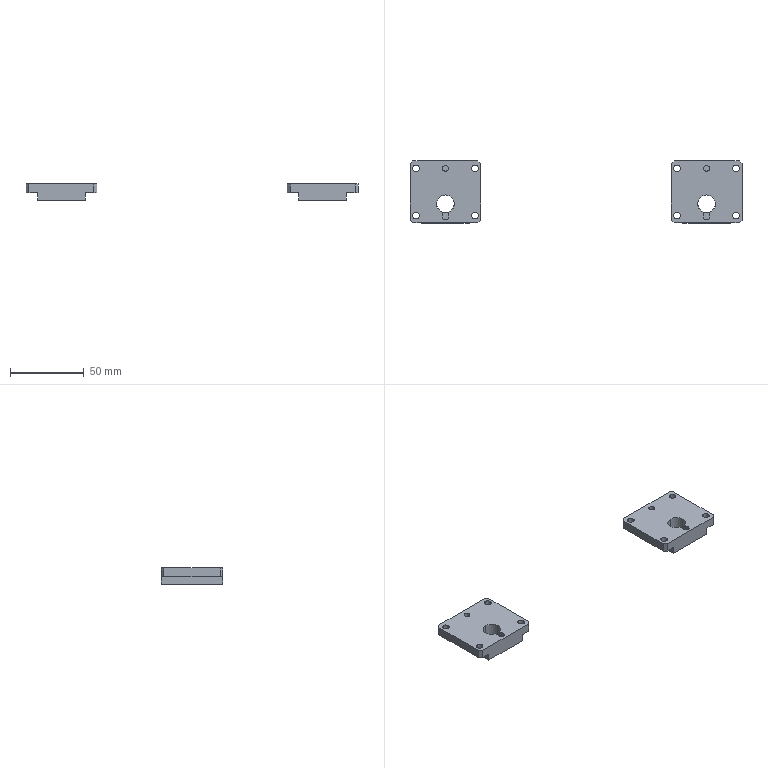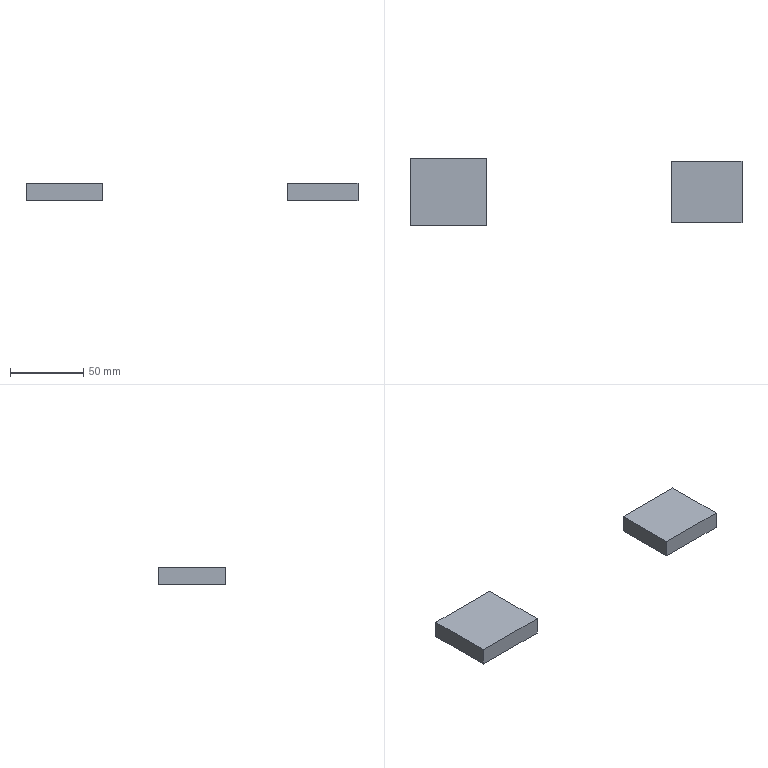CAM job | NX | 3-axis milling, drilling | part box 225 x 42 x 11 mm | stock box 227 x 46 x 12 mm
Tools:
number,name,description,diameter,corner_radius,flute_length,length,flutes
1,D63,Milling Tool-5 Parameters,63.0,0.0,50.0,75.0,2
7,D6A45,Milling Tool-5 Parameters,6.0,0.0,50.0,75.0,2
14,4.5ZT,Drilling Tool,4.5,0.0,35.0,50.0,2
11,D10JING,Milling Tool-5 Parameters,10.0,0.0,50.0,75.0,2
10,D10,Milling Tool-5 Parameters,10.0,0.0,50.0,75.0,2
3,D3,Milling Tool-5 Parameters,3.0,0.0,50.0,75.0,2
12,2.5ZT,Drilling Tool,2.5,0.0,35.0,50.0,2
Operations:
program,operation,operation_type,tool,method,geometry_group,spindle_rpm,surface_speed,feed_per_tooth,feed_cut,feed_plunge,cut_length_mm,path_length_mm,cut_time_min,machine_time_min
1,FLOOR_WALL,VolumeBased25DMillingOperation,D63,METHOD,A,6500.0,1286.0,0.1154,1500.0,100.0,127.0,181.0,0.0847,0.0901
1,DRILLING,Operation,D6A45,METHOD,A,5000.0,94.0,0.025,250.0,0.0,20.0,216.728,0.08,0.0997
1,DRILLING_COPY,Operation,4.5ZT,METHOD,A,2000.0,28.0,0.0625,250.0,0.0,47.408,268.209,0.1896,0.2117
1,ZLEVEL_PROFILE,ZLevelMilling,D10,METHOD,A,9500.0,298.0,0.1579,3000.0,1000.0,7725.108,7793.058,2.598,2.605
1,HOLE_MILLING,CylinderMilling,D10,METHOD,A,9500.0,298.0,0.1053,2000.0,100.0,225.557,296.057,0.1128,0.1198
1,CAVITY_MILL_COPY_1,CavityMilling,D10JING,METHOD,A,9500.0,298.0,0.0632,1200.0,1000.0,214.068,293.968,0.179,0.187
1,HOLE_MILLING_COPY,CylinderMilling,D10JING,METHOD,A,9500.0,298.0,0.0632,1200.0,100.0,27.893,98.393,0.0232,0.0303
1,HOLE_MILLING_1,CylinderMilling,D3,METHOD,A,9500.0,89.0,0.0658,1250.0,100.0,112.872,178.372,0.0903,0.0968
1,ZLEVEL_PROFILE_1,ZLevelMilling,D3,METHOD,A,9500.0,89.0,0.0789,1500.0,100.0,530.475,602.475,0.3537,0.3609
1,PLANAR_MILL_COPY_1,PlanarMilling,D6A45,METHOD,A,9500.0,179.0,0.0658,1250.0,100.0,298.406,853.228,0.2387,0.2942
1,刀补,CylinderMilling,D3,METHOD,A,9500.0,89.0,0.0658,1250.0,100.0,15.482,80.982,0.0124,0.0189
1,刀补1,ZLevelMilling,D3,METHOD,A,9500.0,89.0,0.0632,1200.0,100.0,40.191,112.197,0.0335,0.0407
2,FLOOR_WALL_COPY,VolumeBased25DMillingOperation,D63,METHOD,B,6500.0,1286.0,0.1154,1500.0,100.0,123.0,177.0,0.082,0.0874
2,DRILLING_COPY_1,Operation,D6A45,METHOD,B,5000.0,94.0,0.025,250.0,0.0,16.0,130.831,0.064,0.0755
2,DRILLING_COPY_COPY,Operation,2.5ZT,METHOD,B,2000.0,15.0,0.03,120.0,0.0,42.004,182.84,0.35,0.3641
2,FLOOR_WALL_1,VolumeBased25DMillingOperation,D10,METHOD,B,9500.0,298.0,0.1316,2500.0,1000.0,3555.12,4043.244,1.597,1.645
2,FLOOR_WALL_1_COPY,VolumeBased25DMillingOperation,D10JING,METHOD,B,9500.0,298.0,0.0632,1200.0,1000.0,342.23,531.169,0.287,0.3059
2,HOLE_MILLING_1_COPY,CylinderMilling,D3,METHOD,B,9500.0,89.0,0.0658,1250.0,100.0,225.744,380.745,0.1806,0.1961
2,PLANAR_MILL_COPY_1_COPY,PlanarMilling,D6A45,METHOD,B,9500.0,179.0,0.0658,1250.0,100.0,232.392,642.173,0.1859,0.2269
2,PLANAR_MILL_COPY_1_COPY_COPY,PlanarMilling,D6A45,METHOD,B,9500.0,179.0,0.0658,1250.0,100.0,170.561,766.411,0.1364,0.196
2,刀补_COPY,CylinderMilling,D3,METHOD,B,9500.0,89.0,0.0658,1250.0,100.0,30.964,185.964,0.0248,0.0403